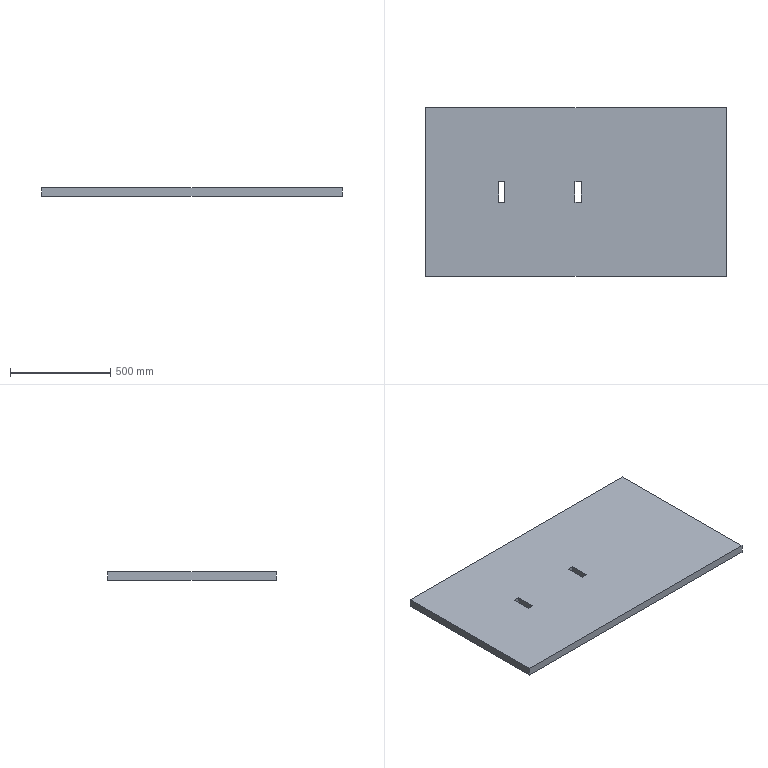Part | SolidWorks | features Extrusion 1 | 1 solid | 14 faces | box 1500 x 840 x 40 mm | volume 50160000 mm3 | plane 14
STEP:
#1=CARTESIAN_POINT('',(365.,470.,40.));
#2=VERTEX_POINT('',#1);
#3=CARTESIAN_POINT('',(365.,370.,40.));
#4=VERTEX_POINT('',#3);
#5=CARTESIAN_POINT('',(365.,470.,40.));
#6=DIRECTION('',(0.,-1.,0.));
#7=VECTOR('',#6,1000.);
#8=LINE('',#5,#7);
#9=EDGE_CURVE('',#2,#4,#8,.T.);
#10=ORIENTED_EDGE('',*,*,#9,.F.);
#11=CARTESIAN_POINT('',(395.,470.,40.));
#12=VERTEX_POINT('',#11);
#13=CARTESIAN_POINT('',(365.,470.,40.));
#14=DIRECTION('',(-1.,0.,0.));
#15=VECTOR('',#14,1000.);
#16=LINE('',#13,#15);
#17=EDGE_CURVE('',#12,#2,#16,.T.);
#18=ORIENTED_EDGE('',*,*,#17,.F.);
#19=CARTESIAN_POINT('',(395.,370.,40.));
#20=VERTEX_POINT('',#19);
#21=CARTESIAN_POINT('',(395.,470.,40.));
#22=DIRECTION('',(0.,1.,0.));
#23=VECTOR('',#22,1000.);
#24=LINE('',#21,#23);
#25=EDGE_CURVE('',#20,#12,#24,.T.);
#26=ORIENTED_EDGE('',*,*,#25,.F.);
#27=CARTESIAN_POINT('',(365.,370.,40.));
#28=DIRECTION('',(1.,0.,0.));
#29=VECTOR('',#28,1000.);
#30=LINE('',#27,#29);
#31=EDGE_CURVE('',#4,#20,#30,.T.);
#32=ORIENTED_EDGE('',*,*,#31,.F.);
#33=EDGE_LOOP('',(#10,#18,#26,#32));
#34=FACE_BOUND('',#33,.T.);
#35=CARTESIAN_POINT('',(0.,840.,40.));
#36=VERTEX_POINT('',#35);
#37=CARTESIAN_POINT('',(0.,0.,40.));
#38=VERTEX_POINT('',#37);
#39=CARTESIAN_POINT('',(0.,0.,40.));
#40=DIRECTION('',(0.,-1.,0.));
#41=VECTOR('',#40,1000.);
#42=LINE('',#39,#41);
#43=EDGE_CURVE('',#36,#38,#42,.T.);
#44=ORIENTED_EDGE('',*,*,#43,.T.);
#45=CARTESIAN_POINT('',(1500.,0.,40.));
#46=VERTEX_POINT('',#45);
#47=CARTESIAN_POINT('',(0.,0.,40.));
#48=DIRECTION('',(1.,0.,0.));
#49=VECTOR('',#48,1000.);
#50=LINE('',#47,#49);
#51=EDGE_CURVE('',#38,#46,#50,.T.);
#52=ORIENTED_EDGE('',*,*,#51,.T.);
#53=CARTESIAN_POINT('',(1500.,840.,40.));
#54=VERTEX_POINT('',#53);
#55=CARTESIAN_POINT('',(1500.,0.,40.));
#56=DIRECTION('',(0.,1.,0.));
#57=VECTOR('',#56,1000.);
#58=LINE('',#55,#57);
#59=EDGE_CURVE('',#46,#54,#58,.T.);
#60=ORIENTED_EDGE('',*,*,#59,.T.);
#61=CARTESIAN_POINT('',(0.,840.,40.));
#62=DIRECTION('',(-1.,0.,0.));
#63=VECTOR('',#62,1000.);
#64=LINE('',#61,#63);
#65=EDGE_CURVE('',#54,#36,#64,.T.);
#66=ORIENTED_EDGE('',*,*,#65,.T.);
#67=EDGE_LOOP('',(#44,#52,#60,#66));
#68=FACE_OUTER_BOUND('',#67,.T.);
#69=CARTESIAN_POINT('',(745.,470.,40.));
#70=VERTEX_POINT('',#69);
#71=CARTESIAN_POINT('',(745.,370.,40.));
#72=VERTEX_POINT('',#71);
#73=CARTESIAN_POINT('',(745.,470.,40.));
#74=DIRECTION('',(0.,-1.,0.));
#75=VECTOR('',#74,1000.);
#76=LINE('',#73,#75);
#77=EDGE_CURVE('',#70,#72,#76,.T.);
#78=ORIENTED_EDGE('',*,*,#77,.F.);
#79=CARTESIAN_POINT('',(775.,470.,40.));
#80=VERTEX_POINT('',#79);
#81=CARTESIAN_POINT('',(745.,470.,40.));
#82=DIRECTION('',(-1.,0.,0.));
#83=VECTOR('',#82,1000.);
#84=LINE('',#81,#83);
#85=EDGE_CURVE('',#80,#70,#84,.T.);
#86=ORIENTED_EDGE('',*,*,#85,.F.);
#87=CARTESIAN_POINT('',(775.,370.,40.));
#88=VERTEX_POINT('',#87);
#89=CARTESIAN_POINT('',(775.,470.,40.));
#90=DIRECTION('',(0.,1.,0.));
#91=VECTOR('',#90,1000.);
#92=LINE('',#89,#91);
#93=EDGE_CURVE('',#88,#80,#92,.T.);
#94=ORIENTED_EDGE('',*,*,#93,.F.);
#95=CARTESIAN_POINT('',(745.,370.,40.));
#96=DIRECTION('',(1.,0.,0.));
#97=VECTOR('',#96,1000.);
#98=LINE('',#95,#97);
#99=EDGE_CURVE('',#72,#88,#98,.T.);
#100=ORIENTED_EDGE('',*,*,#99,.F.);
#101=EDGE_LOOP('',(#78,#86,#94,#100));
#102=FACE_BOUND('',#101,.T.);
#103=CARTESIAN_POINT('',(0.,0.,40.));
#104=DIRECTION('',(0.,0.,-1.));
#105=DIRECTION('',(-1.,0.,0.));
#106=AXIS2_PLACEMENT_3D('',#103,#104,#105);
#107=PLANE('',#106);
#108=ADVANCED_FACE('',(#34,#68,#102),#107,.F.);
#109=CARTESIAN_POINT('',(0.,840.,0.));
#110=VERTEX_POINT('',#109);
#111=CARTESIAN_POINT('',(0.,0.,0.));
#112=VERTEX_POINT('',#111);
#113=CARTESIAN_POINT('',(0.,0.,0.));
#114=DIRECTION('',(0.,-1.,0.));
#115=VECTOR('',#114,1000.);
#116=LINE('',#113,#115);
#117=EDGE_CURVE('',#110,#112,#116,.T.);
#118=ORIENTED_EDGE('',*,*,#117,.F.);
#119=CARTESIAN_POINT('',(1500.,840.,0.));
#120=VERTEX_POINT('',#119);
#121=CARTESIAN_POINT('',(0.,840.,0.));
#122=DIRECTION('',(-1.,0.,0.));
#123=VECTOR('',#122,1000.);
#124=LINE('',#121,#123);
#125=EDGE_CURVE('',#120,#110,#124,.T.);
#126=ORIENTED_EDGE('',*,*,#125,.F.);
#127=CARTESIAN_POINT('',(1500.,0.,0.));
#128=VERTEX_POINT('',#127);
#129=CARTESIAN_POINT('',(1500.,0.,0.));
#130=DIRECTION('',(0.,1.,0.));
#131=VECTOR('',#130,1000.);
#132=LINE('',#129,#131);
#133=EDGE_CURVE('',#128,#120,#132,.T.);
#134=ORIENTED_EDGE('',*,*,#133,.F.);
#135=CARTESIAN_POINT('',(0.,0.,0.));
#136=DIRECTION('',(1.,0.,0.));
#137=VECTOR('',#136,1000.);
#138=LINE('',#135,#137);
#139=EDGE_CURVE('',#112,#128,#138,.T.);
#140=ORIENTED_EDGE('',*,*,#139,.F.);
#141=EDGE_LOOP('',(#118,#126,#134,#140));
#142=FACE_OUTER_BOUND('',#141,.T.);
#143=CARTESIAN_POINT('',(395.,470.,0.));
#144=VERTEX_POINT('',#143);
#145=CARTESIAN_POINT('',(365.,470.,0.));
#146=VERTEX_POINT('',#145);
#147=CARTESIAN_POINT('',(365.,470.,0.));
#148=DIRECTION('',(-1.,0.,0.));
#149=VECTOR('',#148,1000.);
#150=LINE('',#147,#149);
#151=EDGE_CURVE('',#144,#146,#150,.T.);
#152=ORIENTED_EDGE('',*,*,#151,.T.);
#153=CARTESIAN_POINT('',(365.,370.,0.));
#154=VERTEX_POINT('',#153);
#155=CARTESIAN_POINT('',(365.,470.,0.));
#156=DIRECTION('',(0.,-1.,0.));
#157=VECTOR('',#156,1000.);
#158=LINE('',#155,#157);
#159=EDGE_CURVE('',#146,#154,#158,.T.);
#160=ORIENTED_EDGE('',*,*,#159,.T.);
#161=CARTESIAN_POINT('',(395.,370.,0.));
#162=VERTEX_POINT('',#161);
#163=CARTESIAN_POINT('',(365.,370.,0.));
#164=DIRECTION('',(1.,0.,0.));
#165=VECTOR('',#164,1000.);
#166=LINE('',#163,#165);
#167=EDGE_CURVE('',#154,#162,#166,.T.);
#168=ORIENTED_EDGE('',*,*,#167,.T.);
#169=CARTESIAN_POINT('',(395.,470.,0.));
#170=DIRECTION('',(0.,1.,0.));
#171=VECTOR('',#170,1000.);
#172=LINE('',#169,#171);
#173=EDGE_CURVE('',#162,#144,#172,.T.);
#174=ORIENTED_EDGE('',*,*,#173,.T.);
#175=EDGE_LOOP('',(#152,#160,#168,#174));
#176=FACE_BOUND('',#175,.T.);
#177=CARTESIAN_POINT('',(775.,470.,0.));
#178=VERTEX_POINT('',#177);
#179=CARTESIAN_POINT('',(745.,470.,0.));
#180=VERTEX_POINT('',#179);
#181=CARTESIAN_POINT('',(745.,470.,0.));
#182=DIRECTION('',(-1.,0.,0.));
#183=VECTOR('',#182,1000.);
#184=LINE('',#181,#183);
#185=EDGE_CURVE('',#178,#180,#184,.T.);
#186=ORIENTED_EDGE('',*,*,#185,.T.);
#187=CARTESIAN_POINT('',(745.,370.,0.));
#188=VERTEX_POINT('',#187);
#189=CARTESIAN_POINT('',(745.,470.,0.));
#190=DIRECTION('',(0.,-1.,0.));
#191=VECTOR('',#190,1000.);
#192=LINE('',#189,#191);
#193=EDGE_CURVE('',#180,#188,#192,.T.);
#194=ORIENTED_EDGE('',*,*,#193,.T.);
#195=CARTESIAN_POINT('',(775.,370.,0.));
#196=VERTEX_POINT('',#195);
#197=CARTESIAN_POINT('',(745.,370.,0.));
#198=DIRECTION('',(1.,0.,0.));
#199=VECTOR('',#198,1000.);
#200=LINE('',#197,#199);
#201=EDGE_CURVE('',#188,#196,#200,.T.);
#202=ORIENTED_EDGE('',*,*,#201,.T.);
#203=CARTESIAN_POINT('',(775.,470.,0.));
#204=DIRECTION('',(0.,1.,0.));
#205=VECTOR('',#204,1000.);
#206=LINE('',#203,#205);
#207=EDGE_CURVE('',#196,#178,#206,.T.);
#208=ORIENTED_EDGE('',*,*,#207,.T.);
#209=EDGE_LOOP('',(#186,#194,#202,#208));
#210=FACE_BOUND('',#209,.T.);
#211=CARTESIAN_POINT('',(0.,0.,0.));
#212=DIRECTION('',(0.,0.,-1.));
#213=DIRECTION('',(-1.,0.,0.));
#214=AXIS2_PLACEMENT_3D('',#211,#212,#213);
#215=PLANE('',#214);
#216=ADVANCED_FACE('',(#142,#176,#210),#215,.T.);
#217=ORIENTED_EDGE('',*,*,#117,.T.);
#218=CARTESIAN_POINT('',(0.,0.,40.));
#219=DIRECTION('',(0.,0.,-1.));
#220=VECTOR('',#219,1000.);
#221=LINE('',#218,#220);
#222=EDGE_CURVE('',#38,#112,#221,.T.);
#223=ORIENTED_EDGE('',*,*,#222,.F.);
#224=ORIENTED_EDGE('',*,*,#43,.F.);
#225=CARTESIAN_POINT('',(0.,840.,40.));
#226=DIRECTION('',(0.,0.,-1.));
#227=VECTOR('',#226,1000.);
#228=LINE('',#225,#227);
#229=EDGE_CURVE('',#36,#110,#228,.T.);
#230=ORIENTED_EDGE('',*,*,#229,.T.);
#231=EDGE_LOOP('',(#217,#223,#224,#230));
#232=FACE_OUTER_BOUND('',#231,.T.);
#233=CARTESIAN_POINT('',(0.,0.,40.));
#234=DIRECTION('',(1.,0.,0.));
#235=DIRECTION('',(0.,0.,-1.));
#236=AXIS2_PLACEMENT_3D('',#233,#234,#235);
#237=PLANE('',#236);
#238=ADVANCED_FACE('',(#232),#237,.F.);
#239=ORIENTED_EDGE('',*,*,#139,.T.);
#240=CARTESIAN_POINT('',(1500.,0.,40.));
#241=DIRECTION('',(0.,0.,-1.));
#242=VECTOR('',#241,1000.);
#243=LINE('',#240,#242);
#244=EDGE_CURVE('',#46,#128,#243,.T.);
#245=ORIENTED_EDGE('',*,*,#244,.F.);
#246=ORIENTED_EDGE('',*,*,#51,.F.);
#247=ORIENTED_EDGE('',*,*,#222,.T.);
#248=EDGE_LOOP('',(#239,#245,#246,#247));
#249=FACE_OUTER_BOUND('',#248,.T.);
#250=CARTESIAN_POINT('',(0.,0.,40.));
#251=DIRECTION('',(0.,1.,0.));
#252=DIRECTION('',(0.,0.,1.));
#253=AXIS2_PLACEMENT_3D('',#250,#251,#252);
#254=PLANE('',#253);
#255=ADVANCED_FACE('',(#249),#254,.F.);
#256=ORIENTED_EDGE('',*,*,#133,.T.);
#257=CARTESIAN_POINT('',(1500.,840.,40.));
#258=DIRECTION('',(0.,0.,-1.));
#259=VECTOR('',#258,1000.);
#260=LINE('',#257,#259);
#261=EDGE_CURVE('',#54,#120,#260,.T.);
#262=ORIENTED_EDGE('',*,*,#261,.F.);
#263=ORIENTED_EDGE('',*,*,#59,.F.);
#264=ORIENTED_EDGE('',*,*,#244,.T.);
#265=EDGE_LOOP('',(#256,#262,#263,#264));
#266=FACE_OUTER_BOUND('',#265,.T.);
#267=CARTESIAN_POINT('',(1500.,0.,40.));
#268=DIRECTION('',(-1.,0.,0.));
#269=DIRECTION('',(0.,0.,1.));
#270=AXIS2_PLACEMENT_3D('',#267,#268,#269);
#271=PLANE('',#270);
#272=ADVANCED_FACE('',(#266),#271,.F.);
#273=ORIENTED_EDGE('',*,*,#125,.T.);
#274=ORIENTED_EDGE('',*,*,#229,.F.);
#275=ORIENTED_EDGE('',*,*,#65,.F.);
#276=ORIENTED_EDGE('',*,*,#261,.T.);
#277=EDGE_LOOP('',(#273,#274,#275,#276));
#278=FACE_OUTER_BOUND('',#277,.T.);
#279=CARTESIAN_POINT('',(0.,840.,40.));
#280=DIRECTION('',(0.,-1.,0.));
#281=DIRECTION('',(0.,0.,-1.));
#282=AXIS2_PLACEMENT_3D('',#279,#280,#281);
#283=PLANE('',#282);
#284=ADVANCED_FACE('',(#278),#283,.F.);
#285=ORIENTED_EDGE('',*,*,#159,.F.);
#286=CARTESIAN_POINT('',(365.,470.,40.));
#287=DIRECTION('',(0.,0.,-1.));
#288=VECTOR('',#287,1000.);
#289=LINE('',#286,#288);
#290=EDGE_CURVE('',#2,#146,#289,.T.);
#291=ORIENTED_EDGE('',*,*,#290,.F.);
#292=ORIENTED_EDGE('',*,*,#9,.T.);
#293=CARTESIAN_POINT('',(365.,370.,40.));
#294=DIRECTION('',(0.,0.,-1.));
#295=VECTOR('',#294,1000.);
#296=LINE('',#293,#295);
#297=EDGE_CURVE('',#4,#154,#296,.T.);
#298=ORIENTED_EDGE('',*,*,#297,.T.);
#299=EDGE_LOOP('',(#285,#291,#292,#298));
#300=FACE_OUTER_BOUND('',#299,.T.);
#301=CARTESIAN_POINT('',(365.,470.,40.));
#302=DIRECTION('',(1.,0.,0.));
#303=DIRECTION('',(0.,0.,-1.));
#304=AXIS2_PLACEMENT_3D('',#301,#302,#303);
#305=PLANE('',#304);
#306=ADVANCED_FACE('',(#300),#305,.T.);
#307=ORIENTED_EDGE('',*,*,#167,.F.);
#308=ORIENTED_EDGE('',*,*,#297,.F.);
#309=ORIENTED_EDGE('',*,*,#31,.T.);
#310=CARTESIAN_POINT('',(395.,370.,40.));
#311=DIRECTION('',(0.,0.,-1.));
#312=VECTOR('',#311,1000.);
#313=LINE('',#310,#312);
#314=EDGE_CURVE('',#20,#162,#313,.T.);
#315=ORIENTED_EDGE('',*,*,#314,.T.);
#316=EDGE_LOOP('',(#307,#308,#309,#315));
#317=FACE_OUTER_BOUND('',#316,.T.);
#318=CARTESIAN_POINT('',(365.,370.,40.));
#319=DIRECTION('',(0.,1.,0.));
#320=DIRECTION('',(-1.,0.,0.));
#321=AXIS2_PLACEMENT_3D('',#318,#319,#320);
#322=PLANE('',#321);
#323=ADVANCED_FACE('',(#317),#322,.T.);
#324=ORIENTED_EDGE('',*,*,#173,.F.);
#325=ORIENTED_EDGE('',*,*,#314,.F.);
#326=ORIENTED_EDGE('',*,*,#25,.T.);
#327=CARTESIAN_POINT('',(395.,470.,40.));
#328=DIRECTION('',(0.,0.,-1.));
#329=VECTOR('',#328,1000.);
#330=LINE('',#327,#329);
#331=EDGE_CURVE('',#12,#144,#330,.T.);
#332=ORIENTED_EDGE('',*,*,#331,.T.);
#333=EDGE_LOOP('',(#324,#325,#326,#332));
#334=FACE_OUTER_BOUND('',#333,.T.);
#335=CARTESIAN_POINT('',(395.,470.,40.));
#336=DIRECTION('',(-1.,0.,0.));
#337=DIRECTION('',(0.,0.,1.));
#338=AXIS2_PLACEMENT_3D('',#335,#336,#337);
#339=PLANE('',#338);
#340=ADVANCED_FACE('',(#334),#339,.T.);
#341=ORIENTED_EDGE('',*,*,#151,.F.);
#342=ORIENTED_EDGE('',*,*,#331,.F.);
#343=ORIENTED_EDGE('',*,*,#17,.T.);
#344=ORIENTED_EDGE('',*,*,#290,.T.);
#345=EDGE_LOOP('',(#341,#342,#343,#344));
#346=FACE_OUTER_BOUND('',#345,.T.);
#347=CARTESIAN_POINT('',(365.,470.,40.));
#348=DIRECTION('',(0.,-1.,0.));
#349=DIRECTION('',(0.,0.,-1.));
#350=AXIS2_PLACEMENT_3D('',#347,#348,#349);
#351=PLANE('',#350);
#352=ADVANCED_FACE('',(#346),#351,.T.);
#353=ORIENTED_EDGE('',*,*,#193,.F.);
#354=CARTESIAN_POINT('',(745.,470.,40.));
#355=DIRECTION('',(0.,0.,-1.));
#356=VECTOR('',#355,1000.);
#357=LINE('',#354,#356);
#358=EDGE_CURVE('',#70,#180,#357,.T.);
#359=ORIENTED_EDGE('',*,*,#358,.F.);
#360=ORIENTED_EDGE('',*,*,#77,.T.);
#361=CARTESIAN_POINT('',(745.,370.,40.));
#362=DIRECTION('',(0.,0.,-1.));
#363=VECTOR('',#362,1000.);
#364=LINE('',#361,#363);
#365=EDGE_CURVE('',#72,#188,#364,.T.);
#366=ORIENTED_EDGE('',*,*,#365,.T.);
#367=EDGE_LOOP('',(#353,#359,#360,#366));
#368=FACE_OUTER_BOUND('',#367,.T.);
#369=CARTESIAN_POINT('',(745.,470.,40.));
#370=DIRECTION('',(1.,0.,0.));
#371=DIRECTION('',(0.,1.,0.));
#372=AXIS2_PLACEMENT_3D('',#369,#370,#371);
#373=PLANE('',#372);
#374=ADVANCED_FACE('',(#368),#373,.T.);
#375=ORIENTED_EDGE('',*,*,#201,.F.);
#376=ORIENTED_EDGE('',*,*,#365,.F.);
#377=ORIENTED_EDGE('',*,*,#99,.T.);
#378=CARTESIAN_POINT('',(775.,370.,40.));
#379=DIRECTION('',(0.,0.,-1.));
#380=VECTOR('',#379,1000.);
#381=LINE('',#378,#380);
#382=EDGE_CURVE('',#88,#196,#381,.T.);
#383=ORIENTED_EDGE('',*,*,#382,.T.);
#384=EDGE_LOOP('',(#375,#376,#377,#383));
#385=FACE_OUTER_BOUND('',#384,.T.);
#386=CARTESIAN_POINT('',(745.,370.,40.));
#387=DIRECTION('',(0.,1.,0.));
#388=DIRECTION('',(-1.,0.,0.));
#389=AXIS2_PLACEMENT_3D('',#386,#387,#388);
#390=PLANE('',#389);
#391=ADVANCED_FACE('',(#385),#390,.T.);
#392=ORIENTED_EDGE('',*,*,#207,.F.);
#393=ORIENTED_EDGE('',*,*,#382,.F.);
#394=ORIENTED_EDGE('',*,*,#93,.T.);
#395=CARTESIAN_POINT('',(775.,470.,40.));
#396=DIRECTION('',(0.,0.,-1.));
#397=VECTOR('',#396,1000.);
#398=LINE('',#395,#397);
#399=EDGE_CURVE('',#80,#178,#398,.T.);
#400=ORIENTED_EDGE('',*,*,#399,.T.);
#401=EDGE_LOOP('',(#392,#393,#394,#400));
#402=FACE_OUTER_BOUND('',#401,.T.);
#403=CARTESIAN_POINT('',(775.,470.,40.));
#404=DIRECTION('',(-1.,0.,0.));
#405=DIRECTION('',(0.,-1.,0.));
#406=AXIS2_PLACEMENT_3D('',#403,#404,#405);
#407=PLANE('',#406);
#408=ADVANCED_FACE('',(#402),#407,.T.);
#409=ORIENTED_EDGE('',*,*,#185,.F.);
#410=ORIENTED_EDGE('',*,*,#399,.F.);
#411=ORIENTED_EDGE('',*,*,#85,.T.);
#412=ORIENTED_EDGE('',*,*,#358,.T.);
#413=EDGE_LOOP('',(#409,#410,#411,#412));
#414=FACE_OUTER_BOUND('',#413,.T.);
#415=CARTESIAN_POINT('',(745.,470.,40.));
#416=DIRECTION('',(0.,-1.,0.));
#417=DIRECTION('',(0.,0.,-1.));
#418=AXIS2_PLACEMENT_3D('',#415,#416,#417);
#419=PLANE('',#418);
#420=ADVANCED_FACE('',(#414),#419,.T.);
#421=CLOSED_SHELL('',(#108,#216,#238,#255,#272,#284,#306,#323,#340,#352,#374,#391,#408,#420));
#422=MANIFOLD_SOLID_BREP('',#421);
#423=CARTESIAN_POINT('',(0.,0.,0.));
#424=DIRECTION('',(0.,0.,1.));
#425=DIRECTION('',(1.,0.,0.));
#426=AXIS2_PLACEMENT_3D('',#423,#424,#425);
#427=(LENGTH_UNIT()NAMED_UNIT(*)SI_UNIT(.MILLI.,.METRE.));
#428=UNCERTAINTY_MEASURE_WITH_UNIT(LENGTH_MEASURE(0.00001),#427,'','');
#429=(NAMED_UNIT(*)PLANE_ANGLE_UNIT()SI_UNIT($,.RADIAN.));
#430=(NAMED_UNIT(*)SI_UNIT($,.STERADIAN.)SOLID_ANGLE_UNIT());
#431=(GEOMETRIC_REPRESENTATION_CONTEXT(3)GLOBAL_UNCERTAINTY_ASSIGNED_CONTEXT((#428))GLOBAL_UNIT_ASSIGNED_CONTEXT((#427,#429,#430))REPRESENTATION_CONTEXT('',''));
#432=ADVANCED_BREP_SHAPE_REPRESENTATION('',(#422,#426),#431);